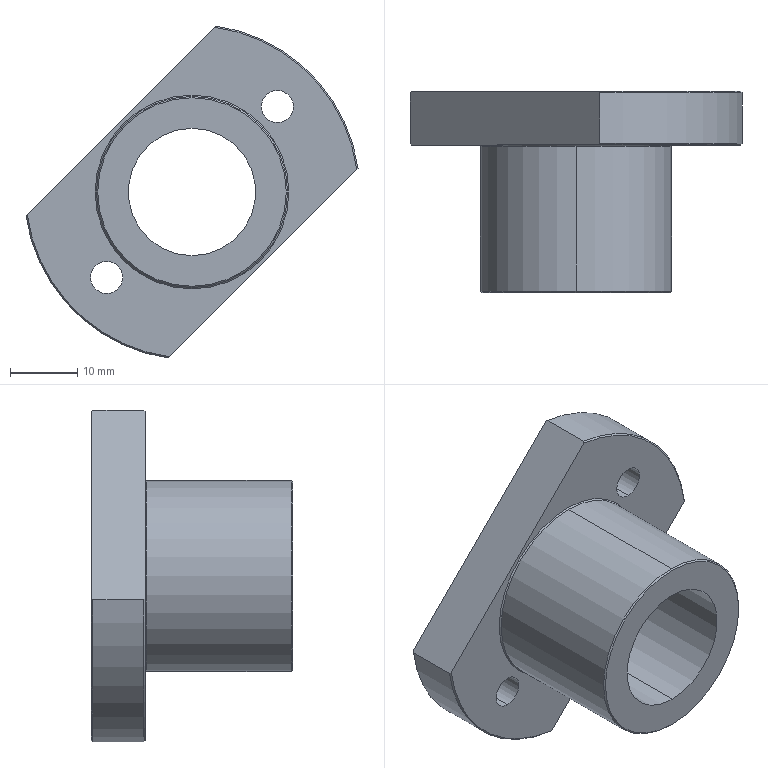Part | SolidWorks | features 3DProfileFeature 2, Chamfer 2, HoleWzd 2, ICE 1, Revolution 1 | 1 solid | 29 faces | box 49.497 x 30 x 49.497 mm | volume 16176 mm3 | cylinder 14 | cone 8 | plane 7 | commonest cylinder face diameters 4.8 x4 8 x4 19 x2 28.5 x2 50 x2
STEP:
#1=CARTESIAN_POINT('',(0.,21.8,-14.25));
#2=VERTEX_POINT('',#1);
#3=CARTESIAN_POINT('',(0.,21.8,14.25));
#4=VERTEX_POINT('',#3);
#5=CARTESIAN_POINT('',(0.,21.8,0.));
#6=DIRECTION('',(0.,-1.,0.));
#7=DIRECTION('',(0.,0.,1.));
#8=AXIS2_PLACEMENT_3D('',#5,#6,#7);
#9=CIRCLE('',#8,14.25);
#10=EDGE_CURVE('',#2,#4,#9,.T.);
#11=ORIENTED_EDGE('',*,*,#10,.F.);
#12=CARTESIAN_POINT('',(0.,22.,-14.45));
#13=VERTEX_POINT('',#12);
#14=CARTESIAN_POINT('',(0.,21.8,-14.25));
#15=DIRECTION('',(0.,0.7071,-0.7071));
#16=VECTOR('',#15,1000.);
#17=LINE('',#14,#16);
#18=EDGE_CURVE('',#2,#13,#17,.T.);
#19=ORIENTED_EDGE('',*,*,#18,.T.);
#20=CARTESIAN_POINT('',(0.,22.,14.45));
#21=VERTEX_POINT('',#20);
#22=CARTESIAN_POINT('',(0.,22.,0.));
#23=DIRECTION('',(0.,1.,0.));
#24=DIRECTION('',(0.,0.,1.));
#25=AXIS2_PLACEMENT_3D('',#22,#23,#24);
#26=CIRCLE('',#25,14.45);
#27=EDGE_CURVE('',#21,#13,#26,.T.);
#28=ORIENTED_EDGE('',*,*,#27,.F.);
#29=CARTESIAN_POINT('',(0.,21.8,14.25));
#30=DIRECTION('',(0.,0.7071,0.7071));
#31=VECTOR('',#30,1000.);
#32=LINE('',#29,#31);
#33=EDGE_CURVE('',#4,#21,#32,.T.);
#34=ORIENTED_EDGE('',*,*,#33,.F.);
#35=EDGE_LOOP('',(#11,#19,#28,#34));
#36=FACE_OUTER_BOUND('',#35,.T.);
#37=CARTESIAN_POINT('',(0.,21.8,0.));
#38=DIRECTION('',(0.,1.,0.));
#39=DIRECTION('',(0.,0.,1.));
#40=AXIS2_PLACEMENT_3D('',#37,#38,#39);
#41=CONICAL_SURFACE('',#40,14.25,0.7854);
#42=ADVANCED_FACE('',(#36),#41,.T.);
#43=CARTESIAN_POINT('',(0.,0.,-14.05));
#44=VERTEX_POINT('',#43);
#45=CARTESIAN_POINT('',(0.,0.,14.05));
#46=VERTEX_POINT('',#45);
#47=CARTESIAN_POINT('',(0.,0.,0.));
#48=DIRECTION('',(0.,-1.,0.));
#49=DIRECTION('',(0.,0.,1.));
#50=AXIS2_PLACEMENT_3D('',#47,#48,#49);
#51=CIRCLE('',#50,14.05);
#52=EDGE_CURVE('',#44,#46,#51,.T.);
#53=ORIENTED_EDGE('',*,*,#52,.F.);
#54=CARTESIAN_POINT('',(0.,0.2,-14.25));
#55=VERTEX_POINT('',#54);
#56=CARTESIAN_POINT('',(0.,0.,-14.05));
#57=DIRECTION('',(0.,0.7071,-0.7071));
#58=VECTOR('',#57,1000.);
#59=LINE('',#56,#58);
#60=EDGE_CURVE('',#44,#55,#59,.T.);
#61=ORIENTED_EDGE('',*,*,#60,.T.);
#62=CARTESIAN_POINT('',(0.,0.2,14.25));
#63=VERTEX_POINT('',#62);
#64=CARTESIAN_POINT('',(0.,0.2,0.));
#65=DIRECTION('',(0.,1.,0.));
#66=DIRECTION('',(0.,0.,1.));
#67=AXIS2_PLACEMENT_3D('',#64,#65,#66);
#68=CIRCLE('',#67,14.25);
#69=EDGE_CURVE('',#63,#55,#68,.T.);
#70=ORIENTED_EDGE('',*,*,#69,.F.);
#71=CARTESIAN_POINT('',(0.,0.,14.05));
#72=DIRECTION('',(0.,0.7071,0.7071));
#73=VECTOR('',#72,1000.);
#74=LINE('',#71,#73);
#75=EDGE_CURVE('',#46,#63,#74,.T.);
#76=ORIENTED_EDGE('',*,*,#75,.F.);
#77=EDGE_LOOP('',(#53,#61,#70,#76));
#78=FACE_OUTER_BOUND('',#77,.T.);
#79=CARTESIAN_POINT('',(0.,0.,0.));
#80=DIRECTION('',(0.,1.,0.));
#81=DIRECTION('',(0.,0.,1.));
#82=AXIS2_PLACEMENT_3D('',#79,#80,#81);
#83=CONICAL_SURFACE('',#82,14.05,0.7854);
#84=ADVANCED_FACE('',(#78),#83,.T.);
#85=CARTESIAN_POINT('',(-12.728,25.4,-16.728));
#86=VERTEX_POINT('',#85);
#87=CARTESIAN_POINT('',(-12.728,25.4,-8.728));
#88=VERTEX_POINT('',#87);
#89=CARTESIAN_POINT('',(-12.728,25.4,-12.728));
#90=DIRECTION('',(0.,1.,0.));
#91=DIRECTION('',(0.,0.,1.));
#92=AXIS2_PLACEMENT_3D('',#89,#90,#91);
#93=CIRCLE('',#92,4.);
#94=EDGE_CURVE('',#86,#88,#93,.T.);
#95=ORIENTED_EDGE('',*,*,#94,.F.);
#96=CARTESIAN_POINT('',(-12.728,30.,-16.728));
#97=VERTEX_POINT('',#96);
#98=CARTESIAN_POINT('',(-12.728,30.,-16.728));
#99=DIRECTION('',(0.,1.,0.));
#100=VECTOR('',#99,1000.);
#101=LINE('',#98,#100);
#102=EDGE_CURVE('',#86,#97,#101,.T.);
#103=ORIENTED_EDGE('',*,*,#102,.T.);
#104=CARTESIAN_POINT('',(-12.728,30.,-8.728));
#105=VERTEX_POINT('',#104);
#106=CARTESIAN_POINT('',(-12.728,30.,-12.728));
#107=DIRECTION('',(0.,1.,0.));
#108=DIRECTION('',(0.,0.,1.));
#109=AXIS2_PLACEMENT_3D('',#106,#107,#108);
#110=CIRCLE('',#109,4.);
#111=EDGE_CURVE('',#97,#105,#110,.T.);
#112=ORIENTED_EDGE('',*,*,#111,.T.);
#113=CARTESIAN_POINT('',(-12.728,30.,-8.728));
#114=DIRECTION('',(0.,1.,0.));
#115=VECTOR('',#114,1000.);
#116=LINE('',#113,#115);
#117=EDGE_CURVE('',#88,#105,#116,.T.);
#118=ORIENTED_EDGE('',*,*,#117,.F.);
#119=EDGE_LOOP('',(#95,#103,#112,#118));
#120=FACE_OUTER_BOUND('',#119,.T.);
#121=CARTESIAN_POINT('',(-12.728,30.,-12.728));
#122=DIRECTION('',(0.,1.,0.));
#123=DIRECTION('',(0.,0.,1.));
#124=AXIS2_PLACEMENT_3D('',#121,#122,#123);
#125=CYLINDRICAL_SURFACE('',#124,4.);
#126=ADVANCED_FACE('',(#120),#125,.F.);
#127=CARTESIAN_POINT('',(-12.728,22.,-15.128));
#128=VERTEX_POINT('',#127);
#129=CARTESIAN_POINT('',(-12.728,22.,-10.328));
#130=VERTEX_POINT('',#129);
#131=CARTESIAN_POINT('',(-12.728,22.,-12.728));
#132=DIRECTION('',(0.,1.,0.));
#133=DIRECTION('',(0.,0.,1.));
#134=AXIS2_PLACEMENT_3D('',#131,#132,#133);
#135=CIRCLE('',#134,2.4);
#136=EDGE_CURVE('',#128,#130,#135,.T.);
#137=ORIENTED_EDGE('',*,*,#136,.F.);
#138=CARTESIAN_POINT('',(-12.728,25.4,-15.128));
#139=VERTEX_POINT('',#138);
#140=CARTESIAN_POINT('',(-12.728,30.,-15.128));
#141=DIRECTION('',(0.,1.,0.));
#142=VECTOR('',#141,1000.);
#143=LINE('',#140,#142);
#144=EDGE_CURVE('',#128,#139,#143,.T.);
#145=ORIENTED_EDGE('',*,*,#144,.T.);
#146=CARTESIAN_POINT('',(-12.728,25.4,-10.328));
#147=VERTEX_POINT('',#146);
#148=CARTESIAN_POINT('',(-12.728,25.4,-12.728));
#149=DIRECTION('',(0.,1.,0.));
#150=DIRECTION('',(0.,0.,1.));
#151=AXIS2_PLACEMENT_3D('',#148,#149,#150);
#152=CIRCLE('',#151,2.4);
#153=EDGE_CURVE('',#139,#147,#152,.T.);
#154=ORIENTED_EDGE('',*,*,#153,.T.);
#155=CARTESIAN_POINT('',(-12.728,30.,-10.328));
#156=DIRECTION('',(0.,1.,0.));
#157=VECTOR('',#156,1000.);
#158=LINE('',#155,#157);
#159=EDGE_CURVE('',#130,#147,#158,.T.);
#160=ORIENTED_EDGE('',*,*,#159,.F.);
#161=EDGE_LOOP('',(#137,#145,#154,#160));
#162=FACE_OUTER_BOUND('',#161,.T.);
#163=CARTESIAN_POINT('',(-12.728,30.,-12.728));
#164=DIRECTION('',(0.,1.,0.));
#165=DIRECTION('',(0.,0.,1.));
#166=AXIS2_PLACEMENT_3D('',#163,#164,#165);
#167=CYLINDRICAL_SURFACE('',#166,2.4);
#168=ADVANCED_FACE('',(#162),#167,.F.);
#169=CARTESIAN_POINT('',(12.728,25.4,8.728));
#170=VERTEX_POINT('',#169);
#171=CARTESIAN_POINT('',(12.728,25.4,16.728));
#172=VERTEX_POINT('',#171);
#173=CARTESIAN_POINT('',(12.728,25.4,12.728));
#174=DIRECTION('',(0.,1.,0.));
#175=DIRECTION('',(0.,0.,1.));
#176=AXIS2_PLACEMENT_3D('',#173,#174,#175);
#177=CIRCLE('',#176,4.);
#178=EDGE_CURVE('',#170,#172,#177,.T.);
#179=ORIENTED_EDGE('',*,*,#178,.F.);
#180=CARTESIAN_POINT('',(12.728,30.,8.728));
#181=VERTEX_POINT('',#180);
#182=CARTESIAN_POINT('',(12.728,30.,8.728));
#183=DIRECTION('',(0.,1.,0.));
#184=VECTOR('',#183,1000.);
#185=LINE('',#182,#184);
#186=EDGE_CURVE('',#170,#181,#185,.T.);
#187=ORIENTED_EDGE('',*,*,#186,.T.);
#188=CARTESIAN_POINT('',(12.728,30.,16.728));
#189=VERTEX_POINT('',#188);
#190=CARTESIAN_POINT('',(12.728,30.,12.728));
#191=DIRECTION('',(0.,1.,0.));
#192=DIRECTION('',(0.,0.,1.));
#193=AXIS2_PLACEMENT_3D('',#190,#191,#192);
#194=CIRCLE('',#193,4.);
#195=EDGE_CURVE('',#181,#189,#194,.T.);
#196=ORIENTED_EDGE('',*,*,#195,.T.);
#197=CARTESIAN_POINT('',(12.728,30.,16.728));
#198=DIRECTION('',(0.,1.,0.));
#199=VECTOR('',#198,1000.);
#200=LINE('',#197,#199);
#201=EDGE_CURVE('',#172,#189,#200,.T.);
#202=ORIENTED_EDGE('',*,*,#201,.F.);
#203=EDGE_LOOP('',(#179,#187,#196,#202));
#204=FACE_OUTER_BOUND('',#203,.T.);
#205=CARTESIAN_POINT('',(12.728,30.,12.728));
#206=DIRECTION('',(0.,1.,0.));
#207=DIRECTION('',(0.,0.,1.));
#208=AXIS2_PLACEMENT_3D('',#205,#206,#207);
#209=CYLINDRICAL_SURFACE('',#208,4.);
#210=ADVANCED_FACE('',(#204),#209,.F.);
#211=CARTESIAN_POINT('',(12.728,22.,10.328));
#212=VERTEX_POINT('',#211);
#213=CARTESIAN_POINT('',(12.728,22.,15.128));
#214=VERTEX_POINT('',#213);
#215=CARTESIAN_POINT('',(12.728,22.,12.728));
#216=DIRECTION('',(0.,1.,0.));
#217=DIRECTION('',(0.,0.,1.));
#218=AXIS2_PLACEMENT_3D('',#215,#216,#217);
#219=CIRCLE('',#218,2.4);
#220=EDGE_CURVE('',#212,#214,#219,.T.);
#221=ORIENTED_EDGE('',*,*,#220,.F.);
#222=CARTESIAN_POINT('',(12.728,25.4,10.328));
#223=VERTEX_POINT('',#222);
#224=CARTESIAN_POINT('',(12.728,30.,10.328));
#225=DIRECTION('',(0.,1.,0.));
#226=VECTOR('',#225,1000.);
#227=LINE('',#224,#226);
#228=EDGE_CURVE('',#212,#223,#227,.T.);
#229=ORIENTED_EDGE('',*,*,#228,.T.);
#230=CARTESIAN_POINT('',(12.728,25.4,15.128));
#231=VERTEX_POINT('',#230);
#232=CARTESIAN_POINT('',(12.728,25.4,12.728));
#233=DIRECTION('',(0.,1.,0.));
#234=DIRECTION('',(0.,0.,1.));
#235=AXIS2_PLACEMENT_3D('',#232,#233,#234);
#236=CIRCLE('',#235,2.4);
#237=EDGE_CURVE('',#223,#231,#236,.T.);
#238=ORIENTED_EDGE('',*,*,#237,.T.);
#239=CARTESIAN_POINT('',(12.728,30.,15.128));
#240=DIRECTION('',(0.,1.,0.));
#241=VECTOR('',#240,1000.);
#242=LINE('',#239,#241);
#243=EDGE_CURVE('',#214,#231,#242,.T.);
#244=ORIENTED_EDGE('',*,*,#243,.F.);
#245=EDGE_LOOP('',(#221,#229,#238,#244));
#246=FACE_OUTER_BOUND('',#245,.T.);
#247=CARTESIAN_POINT('',(12.728,30.,12.728));
#248=DIRECTION('',(0.,1.,0.));
#249=DIRECTION('',(0.,0.,1.));
#250=AXIS2_PLACEMENT_3D('',#247,#248,#249);
#251=CYLINDRICAL_SURFACE('',#250,2.4);
#252=ADVANCED_FACE('',(#246),#251,.F.);
#253=CARTESIAN_POINT('',(0.,0.,-9.5));
#254=VERTEX_POINT('',#253);
#255=CARTESIAN_POINT('',(0.,0.,9.5));
#256=VERTEX_POINT('',#255);
#257=CARTESIAN_POINT('',(0.,0.,0.));
#258=DIRECTION('',(0.,1.,0.));
#259=DIRECTION('',(0.,0.,1.));
#260=AXIS2_PLACEMENT_3D('',#257,#258,#259);
#261=CIRCLE('',#260,9.5);
#262=EDGE_CURVE('',#254,#256,#261,.T.);
#263=ORIENTED_EDGE('',*,*,#262,.F.);
#264=CARTESIAN_POINT('',(0.,30.,-9.5));
#265=VERTEX_POINT('',#264);
#266=CARTESIAN_POINT('',(0.,30.,-9.5));
#267=DIRECTION('',(0.,1.,0.));
#268=VECTOR('',#267,1000.);
#269=LINE('',#266,#268);
#270=EDGE_CURVE('',#254,#265,#269,.T.);
#271=ORIENTED_EDGE('',*,*,#270,.T.);
#272=CARTESIAN_POINT('',(0.,30.,9.5));
#273=VERTEX_POINT('',#272);
#274=CARTESIAN_POINT('',(0.,30.,0.));
#275=DIRECTION('',(0.,1.,0.));
#276=DIRECTION('',(0.,0.,1.));
#277=AXIS2_PLACEMENT_3D('',#274,#275,#276);
#278=CIRCLE('',#277,9.5);
#279=EDGE_CURVE('',#265,#273,#278,.T.);
#280=ORIENTED_EDGE('',*,*,#279,.T.);
#281=CARTESIAN_POINT('',(0.,30.,9.5));
#282=DIRECTION('',(0.,1.,0.));
#283=VECTOR('',#282,1000.);
#284=LINE('',#281,#283);
#285=EDGE_CURVE('',#256,#273,#284,.T.);
#286=ORIENTED_EDGE('',*,*,#285,.F.);
#287=EDGE_LOOP('',(#263,#271,#280,#286));
#288=FACE_OUTER_BOUND('',#287,.T.);
#289=CARTESIAN_POINT('',(0.,30.,0.));
#290=DIRECTION('',(0.,1.,0.));
#291=DIRECTION('',(0.,0.,1.));
#292=AXIS2_PLACEMENT_3D('',#289,#290,#291);
#293=CYLINDRICAL_SURFACE('',#292,9.5);
#294=ADVANCED_FACE('',(#288),#293,.F.);
#295=ORIENTED_EDGE('',*,*,#10,.T.);
#296=CARTESIAN_POINT('',(0.,0.,14.25));
#297=DIRECTION('',(0.,-1.,0.));
#298=VECTOR('',#297,1000.);
#299=LINE('',#296,#298);
#300=EDGE_CURVE('',#4,#63,#299,.T.);
#301=ORIENTED_EDGE('',*,*,#300,.T.);
#302=ORIENTED_EDGE('',*,*,#69,.T.);
#303=CARTESIAN_POINT('',(0.,0.,-14.25));
#304=DIRECTION('',(0.,-1.,0.));
#305=VECTOR('',#304,1000.);
#306=LINE('',#303,#305);
#307=EDGE_CURVE('',#2,#55,#306,.T.);
#308=ORIENTED_EDGE('',*,*,#307,.F.);
#309=EDGE_LOOP('',(#295,#301,#302,#308));
#310=FACE_OUTER_BOUND('',#309,.T.);
#311=CARTESIAN_POINT('',(0.,0.,0.));
#312=DIRECTION('',(0.,-1.,0.));
#313=DIRECTION('',(0.,0.,-1.));
#314=AXIS2_PLACEMENT_3D('',#311,#312,#313);
#315=CYLINDRICAL_SURFACE('',#314,14.25);
#316=ADVANCED_FACE('',(#310),#315,.T.);
#317=CARTESIAN_POINT('',(0.,30.,0.));
#318=DIRECTION('',(0.,1.,0.));
#319=DIRECTION('',(0.,0.,1.));
#320=AXIS2_PLACEMENT_3D('',#317,#318,#319);
#321=CIRCLE('',#320,9.5);
#322=EDGE_CURVE('',#273,#265,#321,.T.);
#323=ORIENTED_EDGE('',*,*,#322,.F.);
#324=ORIENTED_EDGE('',*,*,#279,.F.);
#325=EDGE_LOOP('',(#323,#324));
#326=FACE_BOUND('',#325,.T.);
#327=CARTESIAN_POINT('',(12.728,30.,12.728));
#328=DIRECTION('',(0.,1.,0.));
#329=DIRECTION('',(0.,0.,1.));
#330=AXIS2_PLACEMENT_3D('',#327,#328,#329);
#331=CIRCLE('',#330,4.);
#332=EDGE_CURVE('',#189,#181,#331,.T.);
#333=ORIENTED_EDGE('',*,*,#332,.F.);
#334=ORIENTED_EDGE('',*,*,#195,.F.);
#335=EDGE_LOOP('',(#333,#334));
#336=FACE_BOUND('',#335,.T.);
#337=CARTESIAN_POINT('',(-12.728,30.,-12.728));
#338=DIRECTION('',(0.,1.,0.));
#339=DIRECTION('',(0.,0.,1.));
#340=AXIS2_PLACEMENT_3D('',#337,#338,#339);
#341=CIRCLE('',#340,4.);
#342=EDGE_CURVE('',#105,#97,#341,.T.);
#343=ORIENTED_EDGE('',*,*,#342,.F.);
#344=ORIENTED_EDGE('',*,*,#111,.F.);
#345=EDGE_LOOP('',(#343,#344));
#346=FACE_BOUND('',#345,.T.);
#347=CARTESIAN_POINT('',(24.572,30.,3.358));
#348=VERTEX_POINT('',#347);
#349=CARTESIAN_POINT('',(-3.358,30.,-24.572));
#350=VERTEX_POINT('',#349);
#351=CARTESIAN_POINT('',(-24.749,30.,-45.962));
#352=DIRECTION('',(-0.7071,0.,-0.7071));
#353=VECTOR('',#352,1000.);
#354=LINE('',#351,#353);
#355=EDGE_CURVE('',#348,#350,#354,.T.);
#356=ORIENTED_EDGE('',*,*,#355,.T.);
#357=CARTESIAN_POINT('',(-24.572,30.,-3.358));
#358=VERTEX_POINT('',#357);
#359=CARTESIAN_POINT('',(0.,30.,0.));
#360=DIRECTION('',(0.,1.,0.));
#361=DIRECTION('',(0.,0.,-1.));
#362=AXIS2_PLACEMENT_3D('',#359,#360,#361);
#363=CIRCLE('',#362,24.8);
#364=EDGE_CURVE('',#350,#358,#363,.T.);
#365=ORIENTED_EDGE('',*,*,#364,.T.);
#366=CARTESIAN_POINT('',(3.358,30.,24.572));
#367=VERTEX_POINT('',#366);
#368=CARTESIAN_POINT('',(-45.962,30.,-24.749));
#369=DIRECTION('',(0.7071,0.,0.7071));
#370=VECTOR('',#369,1000.);
#371=LINE('',#368,#370);
#372=EDGE_CURVE('',#358,#367,#371,.T.);
#373=ORIENTED_EDGE('',*,*,#372,.T.);
#374=CARTESIAN_POINT('',(0.,30.,0.));
#375=DIRECTION('',(0.,1.,0.));
#376=DIRECTION('',(0.,0.,-1.));
#377=AXIS2_PLACEMENT_3D('',#374,#375,#376);
#378=CIRCLE('',#377,24.8);
#379=EDGE_CURVE('',#367,#348,#378,.T.);
#380=ORIENTED_EDGE('',*,*,#379,.T.);
#381=EDGE_LOOP('',(#356,#365,#373,#380));
#382=FACE_OUTER_BOUND('',#381,.T.);
#383=CARTESIAN_POINT('',(0.,30.,0.));
#384=DIRECTION('',(0.,-1.,0.));
#385=DIRECTION('',(0.,0.,-1.));
#386=AXIS2_PLACEMENT_3D('',#383,#384,#385);
#387=PLANE('',#386);
#388=ADVANCED_FACE('',(#326,#336,#346,#382),#387,.F.);
#389=CARTESIAN_POINT('',(24.749,29.8,3.536));
#390=VERTEX_POINT('',#389);
#391=CARTESIAN_POINT('',(24.749,22.2,3.536));
#392=VERTEX_POINT('',#391);
#393=CARTESIAN_POINT('',(24.749,0.,3.536));
#394=DIRECTION('',(0.,-1.,0.));
#395=VECTOR('',#394,1000.);
#396=LINE('',#393,#395);
#397=EDGE_CURVE('',#390,#392,#396,.T.);
#398=ORIENTED_EDGE('',*,*,#397,.F.);
#399=CARTESIAN_POINT('',(3.536,29.8,24.749));
#400=VERTEX_POINT('',#399);
#401=CARTESIAN_POINT('',(0.,29.8,0.));
#402=DIRECTION('',(0.,-1.,0.));
#403=DIRECTION('',(0.,0.,-1.));
#404=AXIS2_PLACEMENT_3D('',#401,#402,#403);
#405=CIRCLE('',#404,25.);
#406=EDGE_CURVE('',#390,#400,#405,.T.);
#407=ORIENTED_EDGE('',*,*,#406,.T.);
#408=CARTESIAN_POINT('',(3.536,22.2,24.749));
#409=VERTEX_POINT('',#408);
#410=CARTESIAN_POINT('',(3.536,0.,24.749));
#411=DIRECTION('',(0.,1.,0.));
#412=VECTOR('',#411,1000.);
#413=LINE('',#410,#412);
#414=EDGE_CURVE('',#409,#400,#413,.T.);
#415=ORIENTED_EDGE('',*,*,#414,.F.);
#416=CARTESIAN_POINT('',(0.,22.2,0.));
#417=DIRECTION('',(0.,1.,0.));
#418=DIRECTION('',(0.,0.,1.));
#419=AXIS2_PLACEMENT_3D('',#416,#417,#418);
#420=CIRCLE('',#419,25.);
#421=EDGE_CURVE('',#409,#392,#420,.T.);
#422=ORIENTED_EDGE('',*,*,#421,.T.);
#423=EDGE_LOOP('',(#398,#407,#415,#422));
#424=FACE_OUTER_BOUND('',#423,.T.);
#425=CARTESIAN_POINT('',(0.,0.,0.));
#426=DIRECTION('',(0.,-1.,0.));
#427=DIRECTION('',(0.,0.,-1.));
#428=AXIS2_PLACEMENT_3D('',#425,#426,#427);
#429=CYLINDRICAL_SURFACE('',#428,25.);
#430=ADVANCED_FACE('',(#424),#429,.T.);
#431=CARTESIAN_POINT('',(-3.536,22.2,-24.749));
#432=VERTEX_POINT('',#431);
#433=CARTESIAN_POINT('',(-3.536,29.8,-24.749));
#434=VERTEX_POINT('',#433);
#435=CARTESIAN_POINT('',(-3.536,0.,-24.749));
#436=DIRECTION('',(0.,1.,0.));
#437=VECTOR('',#436,1000.);
#438=LINE('',#435,#437);
#439=EDGE_CURVE('',#432,#434,#438,.T.);
#440=ORIENTED_EDGE('',*,*,#439,.F.);
#441=CARTESIAN_POINT('',(-24.749,22.2,-3.536));
#442=VERTEX_POINT('',#441);
#443=CARTESIAN_POINT('',(0.,22.2,0.));
#444=DIRECTION('',(0.,1.,0.));
#445=DIRECTION('',(0.,0.,1.));
#446=AXIS2_PLACEMENT_3D('',#443,#444,#445);
#447=CIRCLE('',#446,25.);
#448=EDGE_CURVE('',#432,#442,#447,.T.);
#449=ORIENTED_EDGE('',*,*,#448,.T.);
#450=CARTESIAN_POINT('',(-24.749,29.8,-3.536));
#451=VERTEX_POINT('',#450);
#452=CARTESIAN_POINT('',(-24.749,0.,-3.536));
#453=DIRECTION('',(0.,-1.,0.));
#454=VECTOR('',#453,1000.);
#455=LINE('',#452,#454);
#456=EDGE_CURVE('',#451,#442,#455,.T.);
#457=ORIENTED_EDGE('',*,*,#456,.F.);
#458=CARTESIAN_POINT('',(0.,29.8,0.));
#459=DIRECTION('',(0.,-1.,0.));
#460=DIRECTION('',(0.,0.,-1.));
#461=AXIS2_PLACEMENT_3D('',#458,#459,#460);
#462=CIRCLE('',#461,25.);
#463=EDGE_CURVE('',#451,#434,#462,.T.);
#464=ORIENTED_EDGE('',*,*,#463,.T.);
#465=EDGE_LOOP('',(#440,#449,#457,#464));
#466=FACE_OUTER_BOUND('',#465,.T.);
#467=CARTESIAN_POINT('',(0.,0.,0.));
#468=DIRECTION('',(0.,-1.,0.));
#469=DIRECTION('',(0.,0.,-1.));
#470=AXIS2_PLACEMENT_3D('',#467,#468,#469);
#471=CYLINDRICAL_SURFACE('',#470,25.);
#472=ADVANCED_FACE('',(#466),#471,.T.);
#473=ORIENTED_EDGE('',*,*,#27,.T.);
#474=CARTESIAN_POINT('',(0.,22.,0.));
#475=DIRECTION('',(0.,1.,0.));
#476=DIRECTION('',(0.,0.,1.));
#477=AXIS2_PLACEMENT_3D('',#474,#475,#476);
#478=CIRCLE('',#477,14.45);
#479=EDGE_CURVE('',#13,#21,#478,.T.);
#480=ORIENTED_EDGE('',*,*,#479,.T.);
#481=EDGE_LOOP('',(#473,#480));
#482=FACE_BOUND('',#481,.T.);
#483=CARTESIAN_POINT('',(-12.728,22.,-12.728));
#484=DIRECTION('',(0.,1.,0.));
#485=DIRECTION('',(0.,0.,1.));
#486=AXIS2_PLACEMENT_3D('',#483,#484,#485);
#487=CIRCLE('',#486,2.4);
#488=EDGE_CURVE('',#130,#128,#487,.T.);
#489=ORIENTED_EDGE('',*,*,#488,.T.);
#490=ORIENTED_EDGE('',*,*,#136,.T.);
#491=EDGE_LOOP('',(#489,#490));
#492=FACE_BOUND('',#491,.T.);
#493=CARTESIAN_POINT('',(12.728,22.,12.728));
#494=DIRECTION('',(0.,1.,0.));
#495=DIRECTION('',(0.,0.,1.));
#496=AXIS2_PLACEMENT_3D('',#493,#494,#495);
#497=CIRCLE('',#496,2.4);
#498=EDGE_CURVE('',#214,#212,#497,.T.);
#499=ORIENTED_EDGE('',*,*,#498,.T.);
#500=ORIENTED_EDGE('',*,*,#220,.T.);
#501=EDGE_LOOP('',(#499,#500));
#502=FACE_BOUND('',#501,.T.);
#503=CARTESIAN_POINT('',(24.572,22.,3.358));
#504=VERTEX_POINT('',#503);
#505=CARTESIAN_POINT('',(-3.358,22.,-24.572));
#506=VERTEX_POINT('',#505);
#507=CARTESIAN_POINT('',(-1.893,22.,-23.107));
#508=DIRECTION('',(-0.7071,0.,-0.7071));
#509=VECTOR('',#508,1000.);
#510=LINE('',#507,#509);
#511=EDGE_CURVE('',#504,#506,#510,.T.);
#512=ORIENTED_EDGE('',*,*,#511,.F.);
#513=CARTESIAN_POINT('',(3.358,22.,24.572));
#514=VERTEX_POINT('',#513);
#515=CARTESIAN_POINT('',(0.,22.,0.));
#516=DIRECTION('',(0.,-1.,0.));
#517=DIRECTION('',(0.,0.,1.));
#518=AXIS2_PLACEMENT_3D('',#515,#516,#517);
#519=CIRCLE('',#518,24.8);
#520=EDGE_CURVE('',#504,#514,#519,.T.);
#521=ORIENTED_EDGE('',*,*,#520,.T.);
#522=CARTESIAN_POINT('',(-24.572,22.,-3.358));
#523=VERTEX_POINT('',#522);
#524=CARTESIAN_POINT('',(-23.107,22.,-1.893));
#525=DIRECTION('',(0.7071,0.,0.7071));
#526=VECTOR('',#525,1000.);
#527=LINE('',#524,#526);
#528=EDGE_CURVE('',#523,#514,#527,.T.);
#529=ORIENTED_EDGE('',*,*,#528,.F.);
#530=CARTESIAN_POINT('',(0.,22.,0.));
#531=DIRECTION('',(0.,-1.,0.));
#532=DIRECTION('',(0.,0.,1.));
#533=AXIS2_PLACEMENT_3D('',#530,#531,#532);
#534=CIRCLE('',#533,24.8);
#535=EDGE_CURVE('',#523,#506,#534,.T.);
#536=ORIENTED_EDGE('',*,*,#535,.T.);
#537=EDGE_LOOP('',(#512,#521,#529,#536));
#538=FACE_OUTER_BOUND('',#537,.T.);
#539=CARTESIAN_POINT('',(-25.,22.,0.));
#540=DIRECTION('',(0.,1.,0.));
#541=DIRECTION('',(0.,0.,1.));
#542=AXIS2_PLACEMENT_3D('',#539,#540,#541);
#543=PLANE('',#542);
#544=ADVANCED_FACE('',(#482,#492,#502,#538),#543,.F.);
#545=ORIENTED_EDGE('',*,*,#448,.F.);
#546=CARTESIAN_POINT('',(-3.536,22.2,-24.749));
#547=CARTESIAN_POINT('',(-3.477,22.133,-24.69));
#548=CARTESIAN_POINT('',(-3.417,22.067,-24.631));
#549=CARTESIAN_POINT('',(-3.358,22.,-24.572));
#550=B_SPLINE_CURVE_WITH_KNOTS('',3,(#546,#547,#548,#549),.UNSPECIFIED.,.F.,.F.,(4,4),(0.06208,0.0624),.UNSPECIFIED.);
#551=EDGE_CURVE('',#432,#506,#550,.T.);
#552=ORIENTED_EDGE('',*,*,#551,.T.);
#553=ORIENTED_EDGE('',*,*,#535,.F.);
#554=CARTESIAN_POINT('',(-24.572,22.,-3.358));
#555=CARTESIAN_POINT('',(-24.631,22.067,-3.417));
#556=CARTESIAN_POINT('',(-24.69,22.133,-3.477));
#557=CARTESIAN_POINT('',(-24.749,22.2,-3.536));
#558=B_SPLINE_CURVE_WITH_KNOTS('',3,(#554,#555,#556,#557),.UNSPECIFIED.,.F.,.F.,(4,4),(0.1073,0.1076),.UNSPECIFIED.);
#559=EDGE_CURVE('',#523,#442,#558,.T.);
#560=ORIENTED_EDGE('',*,*,#559,.T.);
#561=EDGE_LOOP('',(#545,#552,#553,#560));
#562=FACE_OUTER_BOUND('',#561,.T.);
#563=CARTESIAN_POINT('',(0.,22.,0.));
#564=DIRECTION('',(0.,1.,0.));
#565=DIRECTION('',(0.,0.,1.));
#566=AXIS2_PLACEMENT_3D('',#563,#564,#565);
#567=CONICAL_SURFACE('',#566,24.8,0.7854);
#568=ADVANCED_FACE('',(#562),#567,.T.);
#569=ORIENTED_EDGE('',*,*,#520,.F.);
#570=CARTESIAN_POINT('',(24.572,22.,3.358));
#571=CARTESIAN_POINT('',(24.631,22.067,3.417));
#572=CARTESIAN_POINT('',(24.69,22.133,3.477));
#573=CARTESIAN_POINT('',(24.749,22.2,3.536));
#574=B_SPLINE_CURVE_WITH_KNOTS('',3,(#570,#571,#572,#573),.UNSPECIFIED.,.F.,.F.,(4,4),(0.1073,0.1076),.UNSPECIFIED.);
#575=EDGE_CURVE('',#504,#392,#574,.T.);
#576=ORIENTED_EDGE('',*,*,#575,.T.);
#577=ORIENTED_EDGE('',*,*,#421,.F.);
#578=CARTESIAN_POINT('',(3.536,22.2,24.749));
#579=CARTESIAN_POINT('',(3.477,22.133,24.69));
#580=CARTESIAN_POINT('',(3.417,22.067,24.631));
#581=CARTESIAN_POINT('',(3.358,22.,24.572));
#582=B_SPLINE_CURVE_WITH_KNOTS('',3,(#578,#579,#580,#581),.UNSPECIFIED.,.F.,.F.,(4,4),(0.06208,0.0624),.UNSPECIFIED.);
#583=EDGE_CURVE('',#409,#514,#582,.T.);
#584=ORIENTED_EDGE('',*,*,#583,.T.);
#585=EDGE_LOOP('',(#569,#576,#577,#584));
#586=FACE_OUTER_BOUND('',#585,.T.);
#587=CARTESIAN_POINT('',(0.,22.,0.));
#588=DIRECTION('',(0.,1.,0.));
#589=DIRECTION('',(0.,0.,1.));
#590=AXIS2_PLACEMENT_3D('',#587,#588,#589);
#591=CONICAL_SURFACE('',#590,24.8,0.7854);
#592=ADVANCED_FACE('',(#586),#591,.T.);
#593=ORIENTED_EDGE('',*,*,#406,.F.);
#594=CARTESIAN_POINT('',(24.749,29.8,3.536));
#595=CARTESIAN_POINT('',(24.69,29.867,3.477));
#596=CARTESIAN_POINT('',(24.631,29.933,3.417));
#597=CARTESIAN_POINT('',(24.572,30.,3.358));
#598=B_SPLINE_CURVE_WITH_KNOTS('',3,(#594,#595,#596,#597),.UNSPECIFIED.,.F.,.F.,(4,4),(0.06208,0.0624),.UNSPECIFIED.);
#599=EDGE_CURVE('',#390,#348,#598,.T.);
#600=ORIENTED_EDGE('',*,*,#599,.T.);
#601=ORIENTED_EDGE('',*,*,#379,.F.);
#602=CARTESIAN_POINT('',(3.358,30.,24.572));
#603=CARTESIAN_POINT('',(3.417,29.933,24.631));
#604=CARTESIAN_POINT('',(3.477,29.867,24.69));
#605=CARTESIAN_POINT('',(3.536,29.8,24.749));
#606=B_SPLINE_CURVE_WITH_KNOTS('',3,(#602,#603,#604,#605),.UNSPECIFIED.,.F.,.F.,(4,4),(0.1073,0.1076),.UNSPECIFIED.);
#607=EDGE_CURVE('',#367,#400,#606,.T.);
#608=ORIENTED_EDGE('',*,*,#607,.T.);
#609=EDGE_LOOP('',(#593,#600,#601,#608));
#610=FACE_OUTER_BOUND('',#609,.T.);
#611=CARTESIAN_POINT('',(0.,29.8,0.));
#612=DIRECTION('',(0.,-1.,0.));
#613=DIRECTION('',(0.,0.,-1.));
#614=AXIS2_PLACEMENT_3D('',#611,#612,#613);
#615=CONICAL_SURFACE('',#614,25.,0.7854);
#616=ADVANCED_FACE('',(#610),#615,.T.);
#617=ORIENTED_EDGE('',*,*,#364,.F.);
#618=CARTESIAN_POINT('',(-3.358,30.,-24.572));
#619=CARTESIAN_POINT('',(-3.417,29.933,-24.631));
#620=CARTESIAN_POINT('',(-3.477,29.867,-24.69));
#621=CARTESIAN_POINT('',(-3.536,29.8,-24.749));
#622=B_SPLINE_CURVE_WITH_KNOTS('',3,(#618,#619,#620,#621),.UNSPECIFIED.,.F.,.F.,(4,4),(0.1073,0.1076),.UNSPECIFIED.);
#623=EDGE_CURVE('',#350,#434,#622,.T.);
#624=ORIENTED_EDGE('',*,*,#623,.T.);
#625=ORIENTED_EDGE('',*,*,#463,.F.);
#626=CARTESIAN_POINT('',(-24.749,29.8,-3.536));
#627=CARTESIAN_POINT('',(-24.69,29.867,-3.477));
#628=CARTESIAN_POINT('',(-24.631,29.933,-3.417));
#629=CARTESIAN_POINT('',(-24.572,30.,-3.358));
#630=B_SPLINE_CURVE_WITH_KNOTS('',3,(#626,#627,#628,#629),.UNSPECIFIED.,.F.,.F.,(4,4),(0.06208,0.0624),.UNSPECIFIED.);
#631=EDGE_CURVE('',#451,#358,#630,.T.);
#632=ORIENTED_EDGE('',*,*,#631,.T.);
#633=EDGE_LOOP('',(#617,#624,#625,#632));
#634=FACE_OUTER_BOUND('',#633,.T.);
#635=CARTESIAN_POINT('',(0.,29.8,0.));
#636=DIRECTION('',(0.,-1.,0.));
#637=DIRECTION('',(0.,0.,-1.));
#638=AXIS2_PLACEMENT_3D('',#635,#636,#637);
#639=CONICAL_SURFACE('',#638,25.,0.7854);
#640=ADVANCED_FACE('',(#634),#639,.T.);
#641=ORIENTED_EDGE('',*,*,#300,.F.);
#642=CARTESIAN_POINT('',(0.,21.8,0.));
#643=DIRECTION('',(0.,-1.,0.));
#644=DIRECTION('',(0.,0.,1.));
#645=AXIS2_PLACEMENT_3D('',#642,#643,#644);
#646=CIRCLE('',#645,14.25);
#647=EDGE_CURVE('',#4,#2,#646,.T.);
#648=ORIENTED_EDGE('',*,*,#647,.T.);
#649=ORIENTED_EDGE('',*,*,#307,.T.);
#650=CARTESIAN_POINT('',(0.,0.2,0.));
#651=DIRECTION('',(0.,1.,0.));
#652=DIRECTION('',(0.,0.,1.));
#653=AXIS2_PLACEMENT_3D('',#650,#651,#652);
#654=CIRCLE('',#653,14.25);
#655=EDGE_CURVE('',#55,#63,#654,.T.);
#656=ORIENTED_EDGE('',*,*,#655,.T.);
#657=EDGE_LOOP('',(#641,#648,#649,#656));
#658=FACE_OUTER_BOUND('',#657,.T.);
#659=CARTESIAN_POINT('',(0.,0.,0.));
#660=DIRECTION('',(0.,-1.,0.));
#661=DIRECTION('',(0.,0.,-1.));
#662=AXIS2_PLACEMENT_3D('',#659,#660,#661);
#663=CYLINDRICAL_SURFACE('',#662,14.25);
#664=ADVANCED_FACE('',(#658),#663,.T.);
#665=CARTESIAN_POINT('',(0.,0.,0.));
#666=DIRECTION('',(0.,-1.,0.));
#667=DIRECTION('',(0.,0.,1.));
#668=AXIS2_PLACEMENT_3D('',#665,#666,#667);
#669=CIRCLE('',#668,14.05);
#670=EDGE_CURVE('',#46,#44,#669,.T.);
#671=ORIENTED_EDGE('',*,*,#670,.T.);
#672=ORIENTED_EDGE('',*,*,#52,.T.);
#673=EDGE_LOOP('',(#671,#672));
#674=FACE_OUTER_BOUND('',#673,.T.);
#675=CARTESIAN_POINT('',(0.,0.,0.));
#676=DIRECTION('',(0.,1.,0.));
#677=DIRECTION('',(0.,0.,1.));
#678=AXIS2_PLACEMENT_3D('',#675,#676,#677);
#679=CIRCLE('',#678,9.5);
#680=EDGE_CURVE('',#256,#254,#679,.T.);
#681=ORIENTED_EDGE('',*,*,#680,.T.);
#682=ORIENTED_EDGE('',*,*,#262,.T.);
#683=EDGE_LOOP('',(#681,#682));
#684=FACE_BOUND('',#683,.T.);
#685=CARTESIAN_POINT('',(-14.25,0.,0.));
#686=DIRECTION('',(0.,1.,0.));
#687=DIRECTION('',(0.,0.,1.));
#688=AXIS2_PLACEMENT_3D('',#685,#686,#687);
#689=PLANE('',#688);
#690=ADVANCED_FACE('',(#674,#684),#689,.F.);
#691=ORIENTED_EDGE('',*,*,#270,.F.);
#692=ORIENTED_EDGE('',*,*,#680,.F.);
#693=ORIENTED_EDGE('',*,*,#285,.T.);
#694=ORIENTED_EDGE('',*,*,#322,.T.);
#695=EDGE_LOOP('',(#691,#692,#693,#694));
#696=FACE_OUTER_BOUND('',#695,.T.);
#697=CARTESIAN_POINT('',(0.,30.,0.));
#698=DIRECTION('',(0.,1.,0.));
#699=DIRECTION('',(0.,0.,1.));
#700=AXIS2_PLACEMENT_3D('',#697,#698,#699);
#701=CYLINDRICAL_SURFACE('',#700,9.5);
#702=ADVANCED_FACE('',(#696),#701,.F.);
#703=ORIENTED_EDGE('',*,*,#228,.F.);
#704=ORIENTED_EDGE('',*,*,#498,.F.);
#705=ORIENTED_EDGE('',*,*,#243,.T.);
#706=CARTESIAN_POINT('',(12.728,25.4,12.728));
#707=DIRECTION('',(0.,1.,0.));
#708=DIRECTION('',(0.,0.,1.));
#709=AXIS2_PLACEMENT_3D('',#706,#707,#708);
#710=CIRCLE('',#709,2.4);
#711=EDGE_CURVE('',#231,#223,#710,.T.);
#712=ORIENTED_EDGE('',*,*,#711,.T.);
#713=EDGE_LOOP('',(#703,#704,#705,#712));
#714=FACE_OUTER_BOUND('',#713,.T.);
#715=CARTESIAN_POINT('',(12.728,30.,12.728));
#716=DIRECTION('',(0.,1.,0.));
#717=DIRECTION('',(0.,0.,1.));
#718=AXIS2_PLACEMENT_3D('',#715,#716,#717);
#719=CYLINDRICAL_SURFACE('',#718,2.4);
#720=ADVANCED_FACE('',(#714),#719,.F.);
#721=ORIENTED_EDGE('',*,*,#711,.F.);
#722=ORIENTED_EDGE('',*,*,#237,.F.);
#723=EDGE_LOOP('',(#721,#722));
#724=FACE_BOUND('',#723,.T.);
#725=CARTESIAN_POINT('',(12.728,25.4,12.728));
#726=DIRECTION('',(0.,1.,0.));
#727=DIRECTION('',(0.,0.,1.));
#728=AXIS2_PLACEMENT_3D('',#725,#726,#727);
#729=CIRCLE('',#728,4.);
#730=EDGE_CURVE('',#172,#170,#729,.T.);
#731=ORIENTED_EDGE('',*,*,#730,.T.);
#732=ORIENTED_EDGE('',*,*,#178,.T.);
#733=EDGE_LOOP('',(#731,#732));
#734=FACE_OUTER_BOUND('',#733,.T.);
#735=CARTESIAN_POINT('',(15.128,25.4,12.728));
#736=DIRECTION('',(0.,-1.,0.));
#737=DIRECTION('',(0.,0.,-1.));
#738=AXIS2_PLACEMENT_3D('',#735,#736,#737);
#739=PLANE('',#738);
#740=ADVANCED_FACE('',(#724,#734),#739,.F.);
#741=ORIENTED_EDGE('',*,*,#186,.F.);
#742=ORIENTED_EDGE('',*,*,#730,.F.);
#743=ORIENTED_EDGE('',*,*,#201,.T.);
#744=ORIENTED_EDGE('',*,*,#332,.T.);
#745=EDGE_LOOP('',(#741,#742,#743,#744));
#746=FACE_OUTER_BOUND('',#745,.T.);
#747=CARTESIAN_POINT('',(12.728,30.,12.728));
#748=DIRECTION('',(0.,1.,0.));
#749=DIRECTION('',(0.,0.,1.));
#750=AXIS2_PLACEMENT_3D('',#747,#748,#749);
#751=CYLINDRICAL_SURFACE('',#750,4.);
#752=ADVANCED_FACE('',(#746),#751,.F.);
#753=ORIENTED_EDGE('',*,*,#144,.F.);
#754=ORIENTED_EDGE('',*,*,#488,.F.);
#755=ORIENTED_EDGE('',*,*,#159,.T.);
#756=CARTESIAN_POINT('',(-12.728,25.4,-12.728));
#757=DIRECTION('',(0.,1.,0.));
#758=DIRECTION('',(0.,0.,1.));
#759=AXIS2_PLACEMENT_3D('',#756,#757,#758);
#760=CIRCLE('',#759,2.4);
#761=EDGE_CURVE('',#147,#139,#760,.T.);
#762=ORIENTED_EDGE('',*,*,#761,.T.);
#763=EDGE_LOOP('',(#753,#754,#755,#762));
#764=FACE_OUTER_BOUND('',#763,.T.);
#765=CARTESIAN_POINT('',(-12.728,30.,-12.728));
#766=DIRECTION('',(0.,1.,0.));
#767=DIRECTION('',(0.,0.,1.));
#768=AXIS2_PLACEMENT_3D('',#765,#766,#767);
#769=CYLINDRICAL_SURFACE('',#768,2.4);
#770=ADVANCED_FACE('',(#764),#769,.F.);
#771=ORIENTED_EDGE('',*,*,#761,.F.);
#772=ORIENTED_EDGE('',*,*,#153,.F.);
#773=EDGE_LOOP('',(#771,#772));
#774=FACE_BOUND('',#773,.T.);
#775=CARTESIAN_POINT('',(-12.728,25.4,-12.728));
#776=DIRECTION('',(0.,1.,0.));
#777=DIRECTION('',(0.,0.,1.));
#778=AXIS2_PLACEMENT_3D('',#775,#776,#777);
#779=CIRCLE('',#778,4.);
#780=EDGE_CURVE('',#88,#86,#779,.T.);
#781=ORIENTED_EDGE('',*,*,#780,.T.);
#782=ORIENTED_EDGE('',*,*,#94,.T.);
#783=EDGE_LOOP('',(#781,#782));
#784=FACE_OUTER_BOUND('',#783,.T.);
#785=CARTESIAN_POINT('',(-10.328,25.4,-12.728));
#786=DIRECTION('',(0.,-1.,0.));
#787=DIRECTION('',(0.,0.,-1.));
#788=AXIS2_PLACEMENT_3D('',#785,#786,#787);
#789=PLANE('',#788);
#790=ADVANCED_FACE('',(#774,#784),#789,.F.);
#791=ORIENTED_EDGE('',*,*,#102,.F.);
#792=ORIENTED_EDGE('',*,*,#780,.F.);
#793=ORIENTED_EDGE('',*,*,#117,.T.);
#794=ORIENTED_EDGE('',*,*,#342,.T.);
#795=EDGE_LOOP('',(#791,#792,#793,#794));
#796=FACE_OUTER_BOUND('',#795,.T.);
#797=CARTESIAN_POINT('',(-12.728,30.,-12.728));
#798=DIRECTION('',(0.,1.,0.));
#799=DIRECTION('',(0.,0.,1.));
#800=AXIS2_PLACEMENT_3D('',#797,#798,#799);
#801=CYLINDRICAL_SURFACE('',#800,4.);
#802=ADVANCED_FACE('',(#796),#801,.F.);
#803=ORIENTED_EDGE('',*,*,#60,.F.);
#804=ORIENTED_EDGE('',*,*,#670,.F.);
#805=ORIENTED_EDGE('',*,*,#75,.T.);
#806=ORIENTED_EDGE('',*,*,#655,.F.);
#807=EDGE_LOOP('',(#803,#804,#805,#806));
#808=FACE_OUTER_BOUND('',#807,.T.);
#809=CARTESIAN_POINT('',(0.,0.,0.));
#810=DIRECTION('',(0.,1.,0.));
#811=DIRECTION('',(0.,0.,1.));
#812=AXIS2_PLACEMENT_3D('',#809,#810,#811);
#813=CONICAL_SURFACE('',#812,14.05,0.7854);
#814=ADVANCED_FACE('',(#808),#813,.T.);
#815=ORIENTED_EDGE('',*,*,#18,.F.);
#816=ORIENTED_EDGE('',*,*,#647,.F.);
#817=ORIENTED_EDGE('',*,*,#33,.T.);
#818=ORIENTED_EDGE('',*,*,#479,.F.);
#819=EDGE_LOOP('',(#815,#816,#817,#818));
#820=FACE_OUTER_BOUND('',#819,.T.);
#821=CARTESIAN_POINT('',(0.,21.8,0.));
#822=DIRECTION('',(0.,1.,0.));
#823=DIRECTION('',(0.,0.,1.));
#824=AXIS2_PLACEMENT_3D('',#821,#822,#823);
#825=CONICAL_SURFACE('',#824,14.25,0.7854);
#826=ADVANCED_FACE('',(#820),#825,.T.);
#827=ORIENTED_EDGE('',*,*,#456,.T.);
#828=ORIENTED_EDGE('',*,*,#559,.F.);
#829=ORIENTED_EDGE('',*,*,#528,.T.);
#830=ORIENTED_EDGE('',*,*,#583,.F.);
#831=ORIENTED_EDGE('',*,*,#414,.T.);
#832=ORIENTED_EDGE('',*,*,#607,.F.);
#833=ORIENTED_EDGE('',*,*,#372,.F.);
#834=ORIENTED_EDGE('',*,*,#631,.F.);
#835=EDGE_LOOP('',(#827,#828,#829,#830,#831,#832,#833,#834));
#836=FACE_OUTER_BOUND('',#835,.T.);
#837=CARTESIAN_POINT('',(-45.962,-20.,-24.749));
#838=DIRECTION('',(-0.7071,0.,0.7071));
#839=DIRECTION('',(0.7071,0.,0.7071));
#840=AXIS2_PLACEMENT_3D('',#837,#838,#839);
#841=PLANE('',#840);
#842=ADVANCED_FACE('',(#836),#841,.T.);
#843=ORIENTED_EDGE('',*,*,#397,.T.);
#844=ORIENTED_EDGE('',*,*,#575,.F.);
#845=ORIENTED_EDGE('',*,*,#511,.T.);
#846=ORIENTED_EDGE('',*,*,#551,.F.);
#847=ORIENTED_EDGE('',*,*,#439,.T.);
#848=ORIENTED_EDGE('',*,*,#623,.F.);
#849=ORIENTED_EDGE('',*,*,#355,.F.);
#850=ORIENTED_EDGE('',*,*,#599,.F.);
#851=EDGE_LOOP('',(#843,#844,#845,#846,#847,#848,#849,#850));
#852=FACE_OUTER_BOUND('',#851,.T.);
#853=CARTESIAN_POINT('',(-24.749,-20.,-45.962));
#854=DIRECTION('',(0.7071,0.,-0.7071));
#855=DIRECTION('',(-0.7071,0.,-0.7071));
#856=AXIS2_PLACEMENT_3D('',#853,#854,#855);
#857=PLANE('',#856);
#858=ADVANCED_FACE('',(#852),#857,.T.);
#859=CLOSED_SHELL('',(#42,#84,#126,#168,#210,#252,#294,#316,#388,#430,#472,#544,#568,#592,#616,#640,#664,#690,#702,#720,#740,#752,#770,#790,#802,#814,#826,#842,#858));
#860=MANIFOLD_SOLID_BREP('',#859);
#861=CARTESIAN_POINT('',(0.,0.,0.));
#862=DIRECTION('',(0.,0.,1.));
#863=DIRECTION('',(1.,0.,0.));
#864=AXIS2_PLACEMENT_3D('',#861,#862,#863);
#865=(LENGTH_UNIT()NAMED_UNIT(*)SI_UNIT(.MILLI.,.METRE.));
#866=UNCERTAINTY_MEASURE_WITH_UNIT(LENGTH_MEASURE(0.00001),#865,'','');
#867=(NAMED_UNIT(*)PLANE_ANGLE_UNIT()SI_UNIT($,.RADIAN.));
#868=(NAMED_UNIT(*)SI_UNIT($,.STERADIAN.)SOLID_ANGLE_UNIT());
#869=(GEOMETRIC_REPRESENTATION_CONTEXT(3)GLOBAL_UNCERTAINTY_ASSIGNED_CONTEXT((#866))GLOBAL_UNIT_ASSIGNED_CONTEXT((#865,#867,#868))REPRESENTATION_CONTEXT('',''));
#870=ADVANCED_BREP_SHAPE_REPRESENTATION('',(#860,#864),#869);